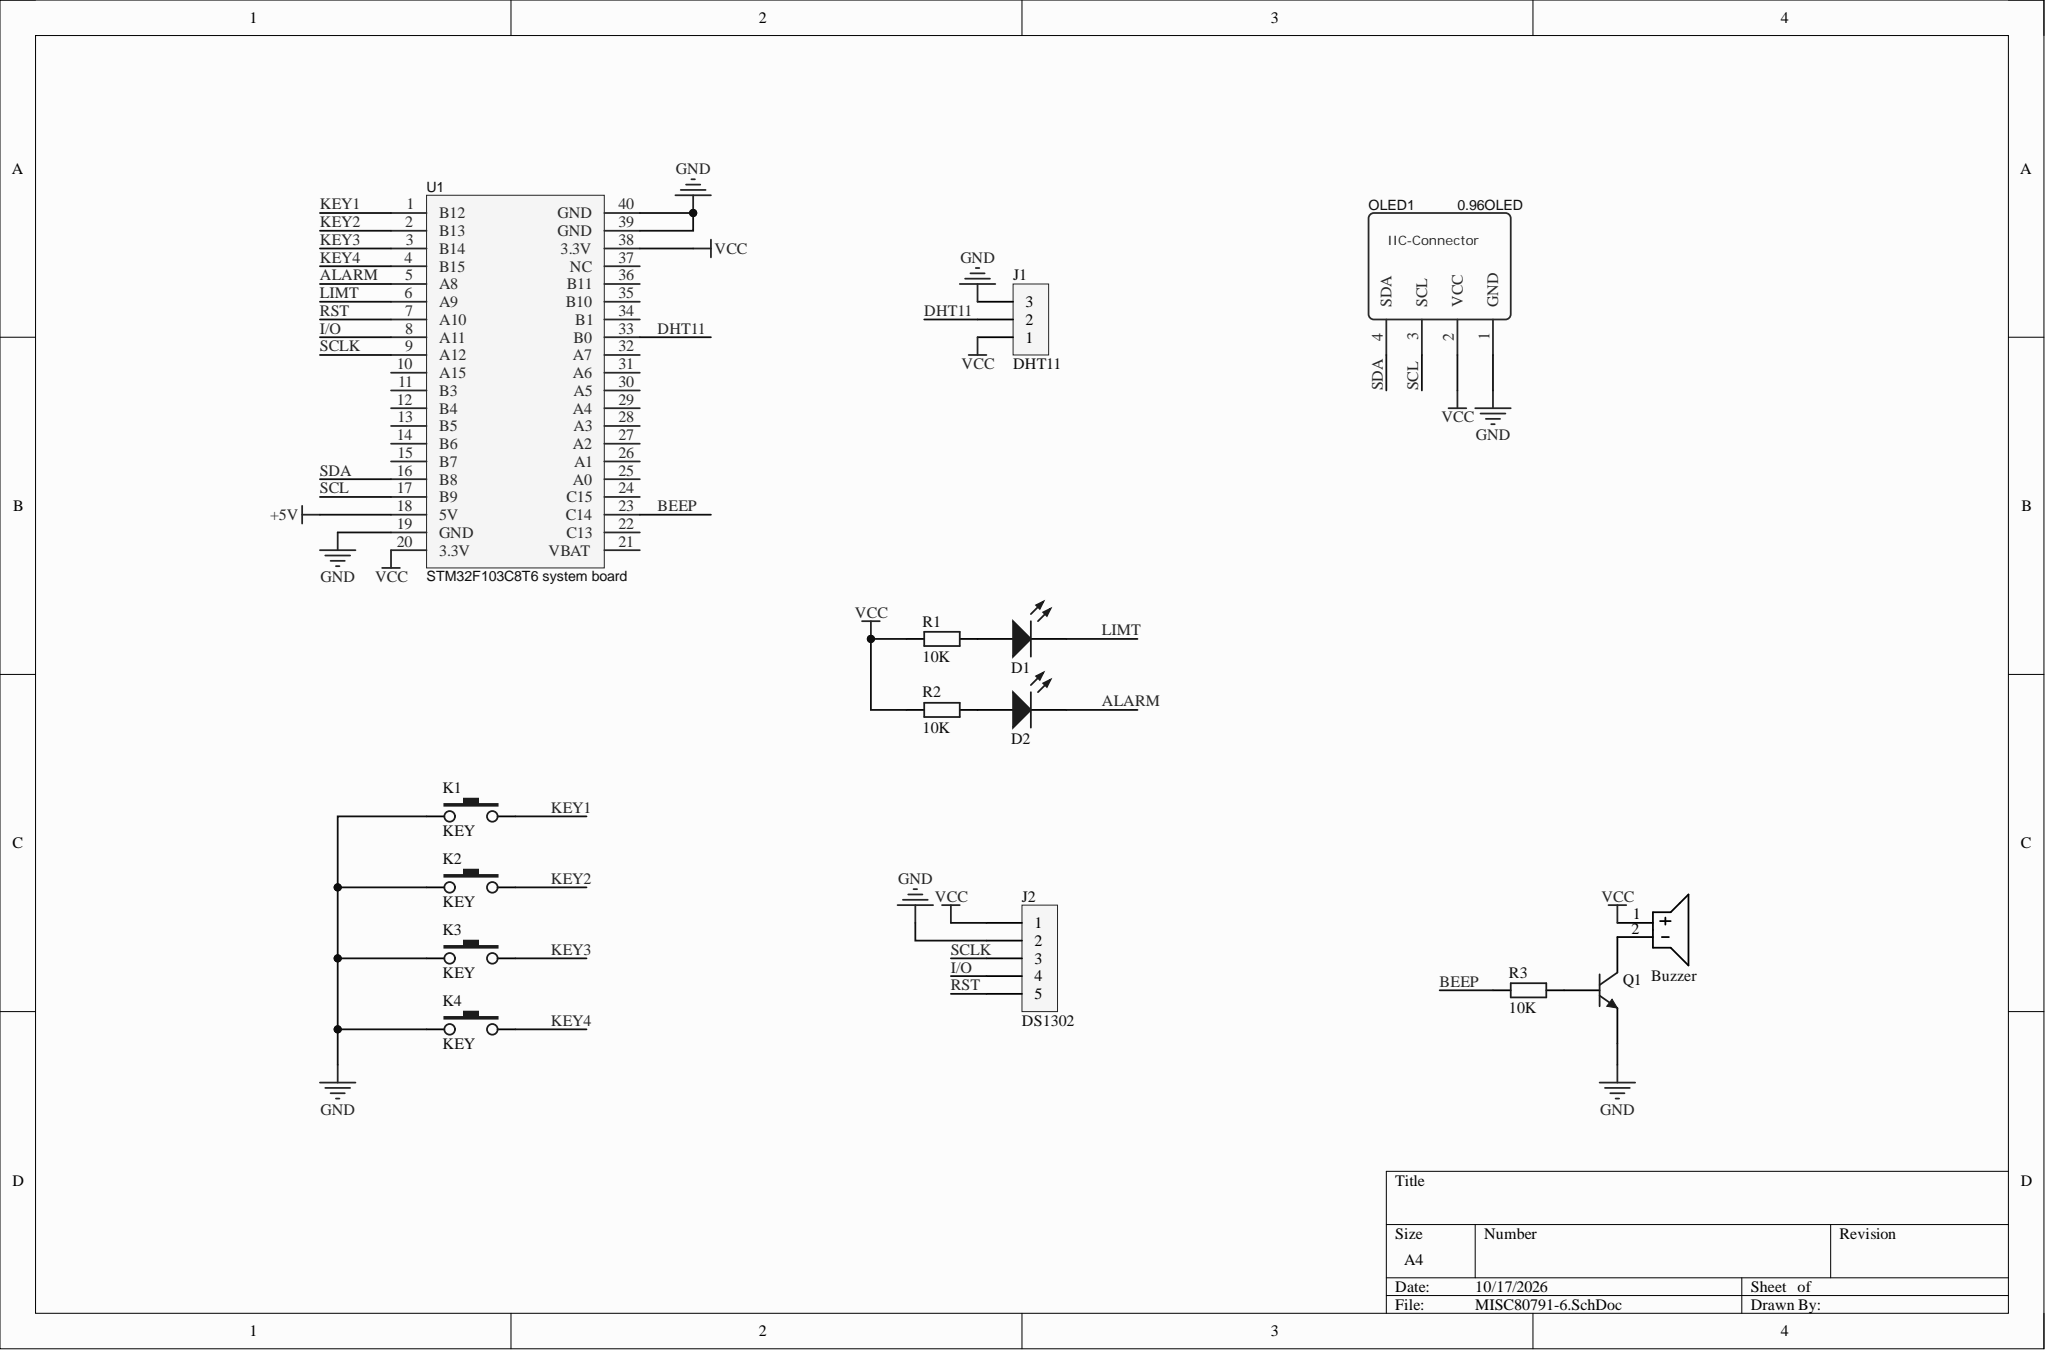Circuit board | Altium Designer | 15 parts | 19 nets
Bill of materials:
Comment,Description,Designator,Footprint,LibRef,Quantity
"Buzzer","","*1","BUZZER","Buzzer","1"
"LED","Light-emitting diode","D1, D2","LED 5MM-W","LED","2"
"DHT11","","J1","Fe-HDR1X3/2.54-S","Female HDR1X3","1"
"DS1302","","J2","Fe-HDR1X5/2.54-S","Female HDR1X5","1"
"KEY","","K1, K2, K3, K4","DIP-3X6X4.3","KEY","4"
"0.96OLED","","OLED1","0.96OLED_4P","0.96OLED_4P_MODULE_JX","1"
"2N3904","NPN General Purpose Amplifier","Q1","TO-92A","2N3904","1"
"10K","Color-band resistor","R1, R2, R3","RS 1/4W","R-S","3"
"STM32F103C8T6 system board","","U1","STM32核心板","STM32F103C8T6系统板","1"
Netlist (Protel format):
[
*1
BUZZER
Buzzer



]
[
D1
LED 5MM-W
LED



]
[
D2
LED 5MM-W
LED



]
[
J1
Fe-HDR1X3/2.54-S
DHT11



]
[
J2
Fe-HDR1X5/2.54-S
DS1302



]
[
K1
DIP-3X6X4.3
KEY



]
[
K2
DIP-3X6X4.3
KEY



]
[
K3
DIP-3X6X4.3
KEY



]
[
K4
DIP-3X6X4.3
KEY



]
[
OLED1
0.96OLED_4P
0.96OLED



]
[
Q1
TO-92A
2N3904



]
[
R1
RS 1/4W
10K



]
[
R2
RS 1/4W
10K



]
[
R3
RS 1/4W
10K



]
[
U1
STM32核心板
STM32F103C8T6 system board



]
(
VCC
*1-1
J1-1
J2-1
OLED1-2
R1-1
R2-1
U1-20
U1-38
)
(
SDA
OLED1-4
U1-16
)
(
SCLK
J2-3
U1-9
)
(
SCL
OLED1-3
U1-17
)
(
RST
J2-5
U1-7
)
(
NetQ1_2
Q1-2
R3-2
)
(
NetD2_1
D2-1
R2-2
)
(
NetD1_1
D1-1
R1-2
)
(
Net*1_2
*1-2
Q1-3
)
(
LIMT
D1-2
U1-6
)
(
KEY4
K4-3
U1-4
)
(
KEY3
K3-3
U1-3
)
(
KEY2
K2-3
U1-2
)
(
KEY1
K1-3
U1-1
)
(
I/O
J2-4
U1-8
)
(
GND
J1-3
J2-2
K1-1
K2-1
K3-1
K4-1
OLED1-1
Q1-1
U1-19
U1-39
U1-40
)
(
DHT11
J1-2
U1-33
)
(
BEEP
R3-1
U1-23
)
(
ALARM
D2-2
U1-5
)